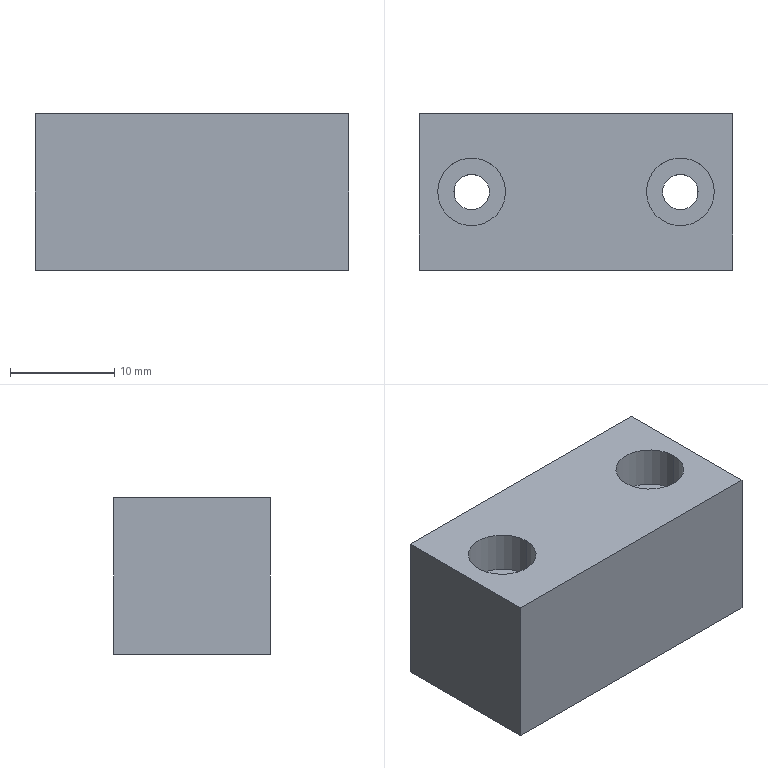Part | STEP file | PN_0020 Default | 1 solid | 16 faces | box 30 x 15 x 15 mm | volume 6285 mm3 | cylinder 8 | plane 8 | commonest cylinder face diameters 3.4 x4 6.5 x4
STEP:
#1=CARTESIAN_POINT('',(-13.25,0.,11.));
#2=VERTEX_POINT('',#1);
#3=CARTESIAN_POINT('',(-6.75,0.,11.));
#4=VERTEX_POINT('',#3);
#5=CARTESIAN_POINT('',(-10.,0.,11.));
#6=DIRECTION('',(0.,0.,1.));
#7=DIRECTION('',(1.,0.,0.));
#8=AXIS2_PLACEMENT_3D('',#5,#6,#7);
#9=CIRCLE('',#8,3.25);
#10=EDGE_CURVE('',#2,#4,#9,.T.);
#11=ORIENTED_EDGE('',*,*,#10,.F.);
#12=CARTESIAN_POINT('',(-13.25,0.,15.));
#13=VERTEX_POINT('',#12);
#14=CARTESIAN_POINT('',(-13.25,0.,15.));
#15=DIRECTION('',(0.,0.,1.));
#16=VECTOR('',#15,1000.);
#17=LINE('',#14,#16);
#18=EDGE_CURVE('',#2,#13,#17,.T.);
#19=ORIENTED_EDGE('',*,*,#18,.T.);
#20=CARTESIAN_POINT('',(-6.75,0.,15.));
#21=VERTEX_POINT('',#20);
#22=CARTESIAN_POINT('',(-10.,0.,15.));
#23=DIRECTION('',(0.,0.,1.));
#24=DIRECTION('',(1.,0.,0.));
#25=AXIS2_PLACEMENT_3D('',#22,#23,#24);
#26=CIRCLE('',#25,3.25);
#27=EDGE_CURVE('',#13,#21,#26,.T.);
#28=ORIENTED_EDGE('',*,*,#27,.T.);
#29=CARTESIAN_POINT('',(-6.75,0.,15.));
#30=DIRECTION('',(0.,0.,1.));
#31=VECTOR('',#30,1000.);
#32=LINE('',#29,#31);
#33=EDGE_CURVE('',#4,#21,#32,.T.);
#34=ORIENTED_EDGE('',*,*,#33,.F.);
#35=EDGE_LOOP('',(#11,#19,#28,#34));
#36=FACE_OUTER_BOUND('',#35,.T.);
#37=CARTESIAN_POINT('',(-10.,0.,15.));
#38=DIRECTION('',(0.,0.,1.));
#39=DIRECTION('',(1.,0.,0.));
#40=AXIS2_PLACEMENT_3D('',#37,#38,#39);
#41=CYLINDRICAL_SURFACE('',#40,3.25);
#42=ADVANCED_FACE('',(#36),#41,.F.);
#43=CARTESIAN_POINT('',(-11.7,0.,0.));
#44=VERTEX_POINT('',#43);
#45=CARTESIAN_POINT('',(-8.3,0.,0.));
#46=VERTEX_POINT('',#45);
#47=CARTESIAN_POINT('',(-10.,0.,0.));
#48=DIRECTION('',(0.,0.,1.));
#49=DIRECTION('',(1.,0.,0.));
#50=AXIS2_PLACEMENT_3D('',#47,#48,#49);
#51=CIRCLE('',#50,1.7);
#52=EDGE_CURVE('',#44,#46,#51,.T.);
#53=ORIENTED_EDGE('',*,*,#52,.F.);
#54=CARTESIAN_POINT('',(-11.7,0.,11.));
#55=VERTEX_POINT('',#54);
#56=CARTESIAN_POINT('',(-11.7,0.,15.));
#57=DIRECTION('',(0.,0.,1.));
#58=VECTOR('',#57,1000.);
#59=LINE('',#56,#58);
#60=EDGE_CURVE('',#44,#55,#59,.T.);
#61=ORIENTED_EDGE('',*,*,#60,.T.);
#62=CARTESIAN_POINT('',(-8.3,0.,11.));
#63=VERTEX_POINT('',#62);
#64=CARTESIAN_POINT('',(-10.,0.,11.));
#65=DIRECTION('',(0.,0.,1.));
#66=DIRECTION('',(1.,0.,0.));
#67=AXIS2_PLACEMENT_3D('',#64,#65,#66);
#68=CIRCLE('',#67,1.7);
#69=EDGE_CURVE('',#55,#63,#68,.T.);
#70=ORIENTED_EDGE('',*,*,#69,.T.);
#71=CARTESIAN_POINT('',(-8.3,0.,15.));
#72=DIRECTION('',(0.,0.,1.));
#73=VECTOR('',#72,1000.);
#74=LINE('',#71,#73);
#75=EDGE_CURVE('',#46,#63,#74,.T.);
#76=ORIENTED_EDGE('',*,*,#75,.F.);
#77=EDGE_LOOP('',(#53,#61,#70,#76));
#78=FACE_OUTER_BOUND('',#77,.T.);
#79=CARTESIAN_POINT('',(-10.,0.,15.));
#80=DIRECTION('',(0.,0.,1.));
#81=DIRECTION('',(1.,0.,0.));
#82=AXIS2_PLACEMENT_3D('',#79,#80,#81);
#83=CYLINDRICAL_SURFACE('',#82,1.7);
#84=ADVANCED_FACE('',(#78),#83,.F.);
#85=CARTESIAN_POINT('',(6.75,0.,11.));
#86=VERTEX_POINT('',#85);
#87=CARTESIAN_POINT('',(13.25,0.,11.));
#88=VERTEX_POINT('',#87);
#89=CARTESIAN_POINT('',(10.,0.,11.));
#90=DIRECTION('',(0.,0.,1.));
#91=DIRECTION('',(1.,0.,0.));
#92=AXIS2_PLACEMENT_3D('',#89,#90,#91);
#93=CIRCLE('',#92,3.25);
#94=EDGE_CURVE('',#86,#88,#93,.T.);
#95=ORIENTED_EDGE('',*,*,#94,.F.);
#96=CARTESIAN_POINT('',(6.75,0.,15.));
#97=VERTEX_POINT('',#96);
#98=CARTESIAN_POINT('',(6.75,0.,15.));
#99=DIRECTION('',(0.,0.,1.));
#100=VECTOR('',#99,1000.);
#101=LINE('',#98,#100);
#102=EDGE_CURVE('',#86,#97,#101,.T.);
#103=ORIENTED_EDGE('',*,*,#102,.T.);
#104=CARTESIAN_POINT('',(13.25,0.,15.));
#105=VERTEX_POINT('',#104);
#106=CARTESIAN_POINT('',(10.,0.,15.));
#107=DIRECTION('',(0.,0.,1.));
#108=DIRECTION('',(1.,0.,0.));
#109=AXIS2_PLACEMENT_3D('',#106,#107,#108);
#110=CIRCLE('',#109,3.25);
#111=EDGE_CURVE('',#97,#105,#110,.T.);
#112=ORIENTED_EDGE('',*,*,#111,.T.);
#113=CARTESIAN_POINT('',(13.25,0.,15.));
#114=DIRECTION('',(0.,0.,1.));
#115=VECTOR('',#114,1000.);
#116=LINE('',#113,#115);
#117=EDGE_CURVE('',#88,#105,#116,.T.);
#118=ORIENTED_EDGE('',*,*,#117,.F.);
#119=EDGE_LOOP('',(#95,#103,#112,#118));
#120=FACE_OUTER_BOUND('',#119,.T.);
#121=CARTESIAN_POINT('',(10.,0.,15.));
#122=DIRECTION('',(0.,0.,1.));
#123=DIRECTION('',(1.,0.,0.));
#124=AXIS2_PLACEMENT_3D('',#121,#122,#123);
#125=CYLINDRICAL_SURFACE('',#124,3.25);
#126=ADVANCED_FACE('',(#120),#125,.F.);
#127=CARTESIAN_POINT('',(8.3,0.,0.));
#128=VERTEX_POINT('',#127);
#129=CARTESIAN_POINT('',(11.7,0.,0.));
#130=VERTEX_POINT('',#129);
#131=CARTESIAN_POINT('',(10.,0.,0.));
#132=DIRECTION('',(0.,0.,1.));
#133=DIRECTION('',(1.,0.,0.));
#134=AXIS2_PLACEMENT_3D('',#131,#132,#133);
#135=CIRCLE('',#134,1.7);
#136=EDGE_CURVE('',#128,#130,#135,.T.);
#137=ORIENTED_EDGE('',*,*,#136,.F.);
#138=CARTESIAN_POINT('',(8.3,0.,11.));
#139=VERTEX_POINT('',#138);
#140=CARTESIAN_POINT('',(8.3,0.,15.));
#141=DIRECTION('',(0.,0.,1.));
#142=VECTOR('',#141,1000.);
#143=LINE('',#140,#142);
#144=EDGE_CURVE('',#128,#139,#143,.T.);
#145=ORIENTED_EDGE('',*,*,#144,.T.);
#146=CARTESIAN_POINT('',(11.7,0.,11.));
#147=VERTEX_POINT('',#146);
#148=CARTESIAN_POINT('',(10.,0.,11.));
#149=DIRECTION('',(0.,0.,1.));
#150=DIRECTION('',(1.,0.,0.));
#151=AXIS2_PLACEMENT_3D('',#148,#149,#150);
#152=CIRCLE('',#151,1.7);
#153=EDGE_CURVE('',#139,#147,#152,.T.);
#154=ORIENTED_EDGE('',*,*,#153,.T.);
#155=CARTESIAN_POINT('',(11.7,0.,15.));
#156=DIRECTION('',(0.,0.,1.));
#157=VECTOR('',#156,1000.);
#158=LINE('',#155,#157);
#159=EDGE_CURVE('',#130,#147,#158,.T.);
#160=ORIENTED_EDGE('',*,*,#159,.F.);
#161=EDGE_LOOP('',(#137,#145,#154,#160));
#162=FACE_OUTER_BOUND('',#161,.T.);
#163=CARTESIAN_POINT('',(10.,0.,15.));
#164=DIRECTION('',(0.,0.,1.));
#165=DIRECTION('',(1.,0.,0.));
#166=AXIS2_PLACEMENT_3D('',#163,#164,#165);
#167=CYLINDRICAL_SURFACE('',#166,1.7);
#168=ADVANCED_FACE('',(#162),#167,.F.);
#169=CARTESIAN_POINT('',(15.,-7.5,0.));
#170=VERTEX_POINT('',#169);
#171=CARTESIAN_POINT('',(15.,7.5,0.));
#172=VERTEX_POINT('',#171);
#173=CARTESIAN_POINT('',(15.,7.5,0.));
#174=DIRECTION('',(0.,1.,0.));
#175=VECTOR('',#174,1000.);
#176=LINE('',#173,#175);
#177=EDGE_CURVE('',#170,#172,#176,.T.);
#178=ORIENTED_EDGE('',*,*,#177,.T.);
#179=CARTESIAN_POINT('',(15.,7.5,15.));
#180=VERTEX_POINT('',#179);
#181=CARTESIAN_POINT('',(15.,7.5,15.));
#182=DIRECTION('',(0.,0.,-1.));
#183=VECTOR('',#182,1000.);
#184=LINE('',#181,#183);
#185=EDGE_CURVE('',#180,#172,#184,.T.);
#186=ORIENTED_EDGE('',*,*,#185,.F.);
#187=CARTESIAN_POINT('',(15.,-7.5,15.));
#188=VERTEX_POINT('',#187);
#189=CARTESIAN_POINT('',(15.,7.5,15.));
#190=DIRECTION('',(0.,1.,0.));
#191=VECTOR('',#190,1000.);
#192=LINE('',#189,#191);
#193=EDGE_CURVE('',#188,#180,#192,.T.);
#194=ORIENTED_EDGE('',*,*,#193,.F.);
#195=CARTESIAN_POINT('',(15.,-7.5,15.));
#196=DIRECTION('',(0.,0.,-1.));
#197=VECTOR('',#196,1000.);
#198=LINE('',#195,#197);
#199=EDGE_CURVE('',#188,#170,#198,.T.);
#200=ORIENTED_EDGE('',*,*,#199,.T.);
#201=EDGE_LOOP('',(#178,#186,#194,#200));
#202=FACE_OUTER_BOUND('',#201,.T.);
#203=CARTESIAN_POINT('',(15.,7.5,15.));
#204=DIRECTION('',(-1.,0.,0.));
#205=DIRECTION('',(0.,-1.,0.));
#206=AXIS2_PLACEMENT_3D('',#203,#204,#205);
#207=PLANE('',#206);
#208=ADVANCED_FACE('',(#202),#207,.F.);
#209=CARTESIAN_POINT('',(-15.,7.5,0.));
#210=VERTEX_POINT('',#209);
#211=CARTESIAN_POINT('',(-15.,7.5,0.));
#212=DIRECTION('',(-1.,0.,0.));
#213=VECTOR('',#212,1000.);
#214=LINE('',#211,#213);
#215=EDGE_CURVE('',#172,#210,#214,.T.);
#216=ORIENTED_EDGE('',*,*,#215,.T.);
#217=CARTESIAN_POINT('',(-15.,7.5,15.));
#218=VERTEX_POINT('',#217);
#219=CARTESIAN_POINT('',(-15.,7.5,15.));
#220=DIRECTION('',(0.,0.,-1.));
#221=VECTOR('',#220,1000.);
#222=LINE('',#219,#221);
#223=EDGE_CURVE('',#218,#210,#222,.T.);
#224=ORIENTED_EDGE('',*,*,#223,.F.);
#225=CARTESIAN_POINT('',(-15.,7.5,15.));
#226=DIRECTION('',(-1.,0.,0.));
#227=VECTOR('',#226,1000.);
#228=LINE('',#225,#227);
#229=EDGE_CURVE('',#180,#218,#228,.T.);
#230=ORIENTED_EDGE('',*,*,#229,.F.);
#231=ORIENTED_EDGE('',*,*,#185,.T.);
#232=EDGE_LOOP('',(#216,#224,#230,#231));
#233=FACE_OUTER_BOUND('',#232,.T.);
#234=CARTESIAN_POINT('',(-15.,7.5,15.));
#235=DIRECTION('',(0.,-1.,0.));
#236=DIRECTION('',(0.,0.,-1.));
#237=AXIS2_PLACEMENT_3D('',#234,#235,#236);
#238=PLANE('',#237);
#239=ADVANCED_FACE('',(#233),#238,.F.);
#240=CARTESIAN_POINT('',(-15.,-7.5,0.));
#241=VERTEX_POINT('',#240);
#242=CARTESIAN_POINT('',(-15.,7.5,0.));
#243=DIRECTION('',(0.,-1.,0.));
#244=VECTOR('',#243,1000.);
#245=LINE('',#242,#244);
#246=EDGE_CURVE('',#210,#241,#245,.T.);
#247=ORIENTED_EDGE('',*,*,#246,.T.);
#248=CARTESIAN_POINT('',(-15.,-7.5,15.));
#249=VERTEX_POINT('',#248);
#250=CARTESIAN_POINT('',(-15.,-7.5,15.));
#251=DIRECTION('',(0.,0.,-1.));
#252=VECTOR('',#251,1000.);
#253=LINE('',#250,#252);
#254=EDGE_CURVE('',#249,#241,#253,.T.);
#255=ORIENTED_EDGE('',*,*,#254,.F.);
#256=CARTESIAN_POINT('',(-15.,7.5,15.));
#257=DIRECTION('',(0.,-1.,0.));
#258=VECTOR('',#257,1000.);
#259=LINE('',#256,#258);
#260=EDGE_CURVE('',#218,#249,#259,.T.);
#261=ORIENTED_EDGE('',*,*,#260,.F.);
#262=ORIENTED_EDGE('',*,*,#223,.T.);
#263=EDGE_LOOP('',(#247,#255,#261,#262));
#264=FACE_OUTER_BOUND('',#263,.T.);
#265=CARTESIAN_POINT('',(-15.,7.5,15.));
#266=DIRECTION('',(1.,0.,0.));
#267=DIRECTION('',(0.,1.,0.));
#268=AXIS2_PLACEMENT_3D('',#265,#266,#267);
#269=PLANE('',#268);
#270=ADVANCED_FACE('',(#264),#269,.F.);
#271=CARTESIAN_POINT('',(-15.,-7.5,0.));
#272=DIRECTION('',(1.,0.,0.));
#273=VECTOR('',#272,1000.);
#274=LINE('',#271,#273);
#275=EDGE_CURVE('',#241,#170,#274,.T.);
#276=ORIENTED_EDGE('',*,*,#275,.T.);
#277=ORIENTED_EDGE('',*,*,#199,.F.);
#278=CARTESIAN_POINT('',(-15.,-7.5,15.));
#279=DIRECTION('',(1.,0.,0.));
#280=VECTOR('',#279,1000.);
#281=LINE('',#278,#280);
#282=EDGE_CURVE('',#249,#188,#281,.T.);
#283=ORIENTED_EDGE('',*,*,#282,.F.);
#284=ORIENTED_EDGE('',*,*,#254,.T.);
#285=EDGE_LOOP('',(#276,#277,#283,#284));
#286=FACE_OUTER_BOUND('',#285,.T.);
#287=CARTESIAN_POINT('',(-15.,-7.5,15.));
#288=DIRECTION('',(0.,1.,0.));
#289=DIRECTION('',(0.,0.,1.));
#290=AXIS2_PLACEMENT_3D('',#287,#288,#289);
#291=PLANE('',#290);
#292=ADVANCED_FACE('',(#286),#291,.F.);
#293=CARTESIAN_POINT('',(-10.,0.,15.));
#294=DIRECTION('',(0.,0.,1.));
#295=DIRECTION('',(1.,0.,0.));
#296=AXIS2_PLACEMENT_3D('',#293,#294,#295);
#297=CIRCLE('',#296,3.25);
#298=EDGE_CURVE('',#21,#13,#297,.T.);
#299=ORIENTED_EDGE('',*,*,#298,.F.);
#300=ORIENTED_EDGE('',*,*,#27,.F.);
#301=EDGE_LOOP('',(#299,#300));
#302=FACE_BOUND('',#301,.T.);
#303=CARTESIAN_POINT('',(10.,0.,15.));
#304=DIRECTION('',(0.,0.,1.));
#305=DIRECTION('',(1.,0.,0.));
#306=AXIS2_PLACEMENT_3D('',#303,#304,#305);
#307=CIRCLE('',#306,3.25);
#308=EDGE_CURVE('',#105,#97,#307,.T.);
#309=ORIENTED_EDGE('',*,*,#308,.F.);
#310=ORIENTED_EDGE('',*,*,#111,.F.);
#311=EDGE_LOOP('',(#309,#310));
#312=FACE_BOUND('',#311,.T.);
#313=ORIENTED_EDGE('',*,*,#193,.T.);
#314=ORIENTED_EDGE('',*,*,#229,.T.);
#315=ORIENTED_EDGE('',*,*,#260,.T.);
#316=ORIENTED_EDGE('',*,*,#282,.T.);
#317=EDGE_LOOP('',(#313,#314,#315,#316));
#318=FACE_OUTER_BOUND('',#317,.T.);
#319=CARTESIAN_POINT('',(0.,0.,15.));
#320=DIRECTION('',(0.,0.,1.));
#321=DIRECTION('',(1.,0.,0.));
#322=AXIS2_PLACEMENT_3D('',#319,#320,#321);
#323=PLANE('',#322);
#324=ADVANCED_FACE('',(#302,#312,#318),#323,.T.);
#325=CARTESIAN_POINT('',(-10.,0.,0.));
#326=DIRECTION('',(0.,0.,1.));
#327=DIRECTION('',(1.,0.,0.));
#328=AXIS2_PLACEMENT_3D('',#325,#326,#327);
#329=CIRCLE('',#328,1.7);
#330=EDGE_CURVE('',#46,#44,#329,.T.);
#331=ORIENTED_EDGE('',*,*,#330,.T.);
#332=ORIENTED_EDGE('',*,*,#52,.T.);
#333=EDGE_LOOP('',(#331,#332));
#334=FACE_BOUND('',#333,.T.);
#335=CARTESIAN_POINT('',(10.,0.,0.));
#336=DIRECTION('',(0.,0.,1.));
#337=DIRECTION('',(1.,0.,0.));
#338=AXIS2_PLACEMENT_3D('',#335,#336,#337);
#339=CIRCLE('',#338,1.7);
#340=EDGE_CURVE('',#130,#128,#339,.T.);
#341=ORIENTED_EDGE('',*,*,#340,.T.);
#342=ORIENTED_EDGE('',*,*,#136,.T.);
#343=EDGE_LOOP('',(#341,#342));
#344=FACE_BOUND('',#343,.T.);
#345=ORIENTED_EDGE('',*,*,#177,.F.);
#346=ORIENTED_EDGE('',*,*,#275,.F.);
#347=ORIENTED_EDGE('',*,*,#246,.F.);
#348=ORIENTED_EDGE('',*,*,#215,.F.);
#349=EDGE_LOOP('',(#345,#346,#347,#348));
#350=FACE_OUTER_BOUND('',#349,.T.);
#351=CARTESIAN_POINT('',(0.,0.,0.));
#352=DIRECTION('',(0.,0.,1.));
#353=DIRECTION('',(1.,0.,0.));
#354=AXIS2_PLACEMENT_3D('',#351,#352,#353);
#355=PLANE('',#354);
#356=ADVANCED_FACE('',(#334,#344,#350),#355,.F.);
#357=ORIENTED_EDGE('',*,*,#144,.F.);
#358=ORIENTED_EDGE('',*,*,#340,.F.);
#359=ORIENTED_EDGE('',*,*,#159,.T.);
#360=CARTESIAN_POINT('',(10.,0.,11.));
#361=DIRECTION('',(0.,0.,1.));
#362=DIRECTION('',(1.,0.,0.));
#363=AXIS2_PLACEMENT_3D('',#360,#361,#362);
#364=CIRCLE('',#363,1.7);
#365=EDGE_CURVE('',#147,#139,#364,.T.);
#366=ORIENTED_EDGE('',*,*,#365,.T.);
#367=EDGE_LOOP('',(#357,#358,#359,#366));
#368=FACE_OUTER_BOUND('',#367,.T.);
#369=CARTESIAN_POINT('',(10.,0.,15.));
#370=DIRECTION('',(0.,0.,1.));
#371=DIRECTION('',(1.,0.,0.));
#372=AXIS2_PLACEMENT_3D('',#369,#370,#371);
#373=CYLINDRICAL_SURFACE('',#372,1.7);
#374=ADVANCED_FACE('',(#368),#373,.F.);
#375=ORIENTED_EDGE('',*,*,#365,.F.);
#376=ORIENTED_EDGE('',*,*,#153,.F.);
#377=EDGE_LOOP('',(#375,#376));
#378=FACE_BOUND('',#377,.T.);
#379=CARTESIAN_POINT('',(10.,0.,11.));
#380=DIRECTION('',(0.,0.,1.));
#381=DIRECTION('',(1.,0.,0.));
#382=AXIS2_PLACEMENT_3D('',#379,#380,#381);
#383=CIRCLE('',#382,3.25);
#384=EDGE_CURVE('',#88,#86,#383,.T.);
#385=ORIENTED_EDGE('',*,*,#384,.T.);
#386=ORIENTED_EDGE('',*,*,#94,.T.);
#387=EDGE_LOOP('',(#385,#386));
#388=FACE_OUTER_BOUND('',#387,.T.);
#389=CARTESIAN_POINT('',(11.7,0.,11.));
#390=DIRECTION('',(0.,0.,-1.));
#391=DIRECTION('',(-1.,0.,0.));
#392=AXIS2_PLACEMENT_3D('',#389,#390,#391);
#393=PLANE('',#392);
#394=ADVANCED_FACE('',(#378,#388),#393,.F.);
#395=ORIENTED_EDGE('',*,*,#102,.F.);
#396=ORIENTED_EDGE('',*,*,#384,.F.);
#397=ORIENTED_EDGE('',*,*,#117,.T.);
#398=ORIENTED_EDGE('',*,*,#308,.T.);
#399=EDGE_LOOP('',(#395,#396,#397,#398));
#400=FACE_OUTER_BOUND('',#399,.T.);
#401=CARTESIAN_POINT('',(10.,0.,15.));
#402=DIRECTION('',(0.,0.,1.));
#403=DIRECTION('',(1.,0.,0.));
#404=AXIS2_PLACEMENT_3D('',#401,#402,#403);
#405=CYLINDRICAL_SURFACE('',#404,3.25);
#406=ADVANCED_FACE('',(#400),#405,.F.);
#407=ORIENTED_EDGE('',*,*,#60,.F.);
#408=ORIENTED_EDGE('',*,*,#330,.F.);
#409=ORIENTED_EDGE('',*,*,#75,.T.);
#410=CARTESIAN_POINT('',(-10.,0.,11.));
#411=DIRECTION('',(0.,0.,1.));
#412=DIRECTION('',(1.,0.,0.));
#413=AXIS2_PLACEMENT_3D('',#410,#411,#412);
#414=CIRCLE('',#413,1.7);
#415=EDGE_CURVE('',#63,#55,#414,.T.);
#416=ORIENTED_EDGE('',*,*,#415,.T.);
#417=EDGE_LOOP('',(#407,#408,#409,#416));
#418=FACE_OUTER_BOUND('',#417,.T.);
#419=CARTESIAN_POINT('',(-10.,0.,15.));
#420=DIRECTION('',(0.,0.,1.));
#421=DIRECTION('',(1.,0.,0.));
#422=AXIS2_PLACEMENT_3D('',#419,#420,#421);
#423=CYLINDRICAL_SURFACE('',#422,1.7);
#424=ADVANCED_FACE('',(#418),#423,.F.);
#425=ORIENTED_EDGE('',*,*,#415,.F.);
#426=ORIENTED_EDGE('',*,*,#69,.F.);
#427=EDGE_LOOP('',(#425,#426));
#428=FACE_BOUND('',#427,.T.);
#429=CARTESIAN_POINT('',(-10.,0.,11.));
#430=DIRECTION('',(0.,0.,1.));
#431=DIRECTION('',(1.,0.,0.));
#432=AXIS2_PLACEMENT_3D('',#429,#430,#431);
#433=CIRCLE('',#432,3.25);
#434=EDGE_CURVE('',#4,#2,#433,.T.);
#435=ORIENTED_EDGE('',*,*,#434,.T.);
#436=ORIENTED_EDGE('',*,*,#10,.T.);
#437=EDGE_LOOP('',(#435,#436));
#438=FACE_OUTER_BOUND('',#437,.T.);
#439=CARTESIAN_POINT('',(-8.3,0.,11.));
#440=DIRECTION('',(0.,0.,-1.));
#441=DIRECTION('',(-1.,0.,0.));
#442=AXIS2_PLACEMENT_3D('',#439,#440,#441);
#443=PLANE('',#442);
#444=ADVANCED_FACE('',(#428,#438),#443,.F.);
#445=ORIENTED_EDGE('',*,*,#18,.F.);
#446=ORIENTED_EDGE('',*,*,#434,.F.);
#447=ORIENTED_EDGE('',*,*,#33,.T.);
#448=ORIENTED_EDGE('',*,*,#298,.T.);
#449=EDGE_LOOP('',(#445,#446,#447,#448));
#450=FACE_OUTER_BOUND('',#449,.T.);
#451=CARTESIAN_POINT('',(-10.,0.,15.));
#452=DIRECTION('',(0.,0.,1.));
#453=DIRECTION('',(1.,0.,0.));
#454=AXIS2_PLACEMENT_3D('',#451,#452,#453);
#455=CYLINDRICAL_SURFACE('',#454,3.25);
#456=ADVANCED_FACE('',(#450),#455,.F.);
#457=CLOSED_SHELL('',(#42,#84,#126,#168,#208,#239,#270,#292,#324,#356,#374,#394,#406,#424,#444,#456));
#458=MANIFOLD_SOLID_BREP('',#457);
#459=CARTESIAN_POINT('',(0.,0.,0.));
#460=DIRECTION('',(0.,0.,1.));
#461=DIRECTION('',(1.,0.,0.));
#462=AXIS2_PLACEMENT_3D('',#459,#460,#461);
#463=(LENGTH_UNIT()NAMED_UNIT(*)SI_UNIT(.MILLI.,.METRE.));
#464=UNCERTAINTY_MEASURE_WITH_UNIT(LENGTH_MEASURE(0.00001),#463,'','');
#465=(NAMED_UNIT(*)PLANE_ANGLE_UNIT()SI_UNIT($,.RADIAN.));
#466=(NAMED_UNIT(*)SI_UNIT($,.STERADIAN.)SOLID_ANGLE_UNIT());
#467=(GEOMETRIC_REPRESENTATION_CONTEXT(3)GLOBAL_UNCERTAINTY_ASSIGNED_CONTEXT((#464))GLOBAL_UNIT_ASSIGNED_CONTEXT((#463,#465,#466))REPRESENTATION_CONTEXT('',''));
#468=ADVANCED_BREP_SHAPE_REPRESENTATION('',(#458,#462),#467);